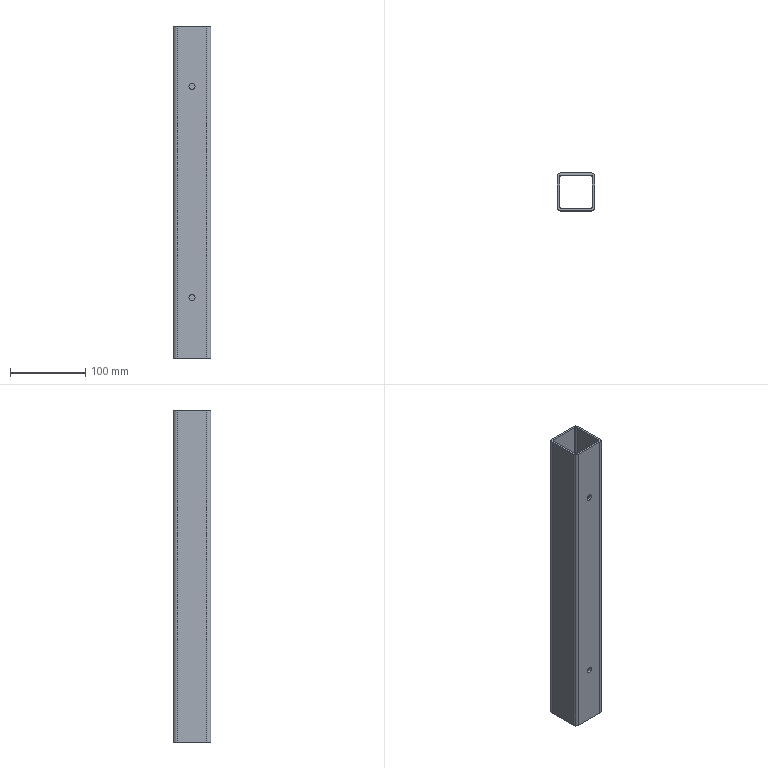Part | STEP file | POST.SQ.PIPE.3.stp | 1 solid | 30 faces | box 50 x 50 x 440 mm | volume 254554 mm3 | cylinder 18 | plane 10 | spline 2 | commonest cylinder face diameters 4 x8 10.4 x8 8 x2